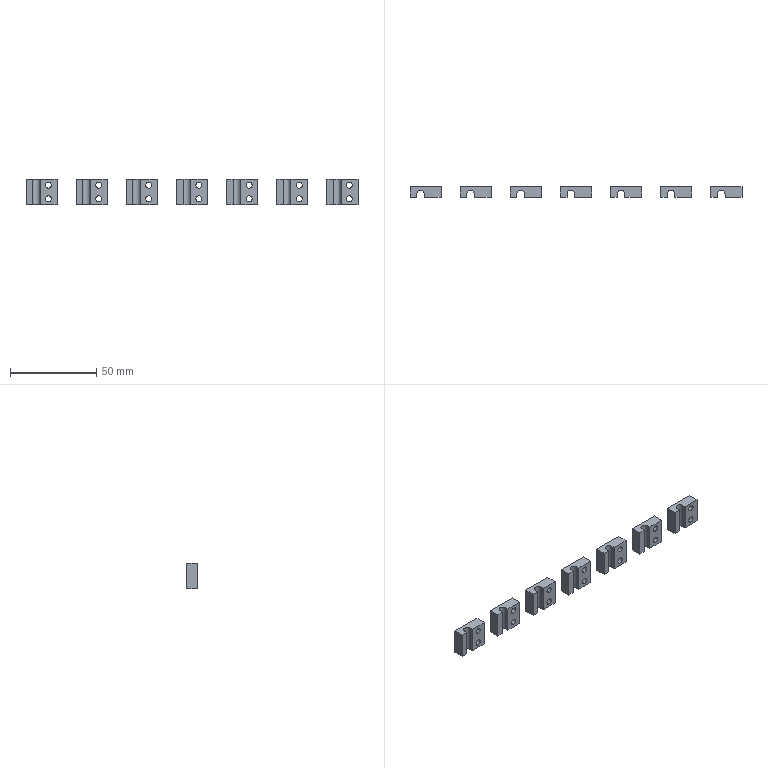NC program | Mastercam | posted with a generic post | part box 192 x 6 x 15 mm
Lines 1 to 1607 of 12453, first 1512 of 1607 lines:
%
:0001()
(MATERIAL - ALUMINUM MM - 2024)
(T20|63 FEM |H20)
(T9|10 FEM |H9|XY STOCK TO LEAVE - .1|Z STOCK TO LEAVE - 0.)
(T10|10 FEM |H10)
(T2|2 FEM |H2)
(T5|3 BM/BNOS |H5)
(T7|4 CHM |H7)
N100 G21
N102 G0 G17 G40 G80 G90 G94 G98
N104 G0 G28 G91 Z0.
N106 G0 G28 X0. Y0.
(63 FEM |TOOL - 20|DIA. OFF. - 20|LEN. - 20|TOOL DIA. - 63.)
N108 T20 M6
N110 G0 G54 G90 X-146.4 Y0. C0. B0. S4000 M3
N112 G43 H20 Z50.
N114 Z2.
N116 G1 Z0. F600.
N118 X146.4 F1000.
N120 G0 Z50.
N122 M5
N124 G0 G28 G91 Z0.
N126 G28
N128 M01
N130 G0 G17 G40 G80 G90 G94 G98
N132 G0 G28 G91 Z0.
(10 FEM |TOOL - 9|DIA. OFF. - 9|LEN. - 9|TOOL DIA. - 10.)
N134 T9 M6
N136 G0 G54 G90 X97. Y-18.6 C0. B0. S10000 M3
N138 G43 H9 Z50.
N140 Z1.
N142 G1 Z0. F600.
N144 Y-13.6 F4000.
N146 G3 X96. Y-12.6 I-1.
N148 G1 X78. Z-.092
N150 G2 X72.9 Y-7.5 Z-.133 J5.1
N152 G1 Y7.5 Z-.209
N154 G2 X78. Y12.6 Z-.25 I5.1
N156 G1 X96. Z-.342
N158 G2 X101.1 Y7.5 Z-.383 J-5.1
N160 G1 Y-7.5 Z-.459
N162 G2 X96. Y-12.6 Z-.5 I-5.1
N164 G1 X78. Z-.592
N166 G2 X72.9 Y-7.5 Z-.633 J5.1
N168 G1 Y7.5 Z-.709
N170 G2 X78. Y12.6 Z-.75 I5.1
N172 G1 X96. Z-.842
N174 G2 X101.1 Y7.5 Z-.883 J-5.1
N176 G1 Y-7.5 Z-.959
N178 G2 X96. Y-12.6 Z-1. I-5.1
N180 G1 X78. Z-1.092
N182 G2 X72.9 Y-7.5 Z-1.133 J5.1
N184 G1 Y7.5 Z-1.209
N186 G2 X78. Y12.6 Z-1.25 I5.1
N188 G1 X96. Z-1.342
N190 G2 X101.1 Y7.5 Z-1.383 J-5.1
N192 G1 Y-7.5 Z-1.459
N194 G2 X96. Y-12.6 Z-1.5 I-5.1
N196 G1 X78. Z-1.592
N198 G2 X72.9 Y-7.5 Z-1.633 J5.1
N200 G1 Y7.5 Z-1.709
N202 G2 X78. Y12.6 Z-1.75 I5.1
N204 G1 X96. Z-1.842
N206 G2 X101.1 Y7.5 Z-1.883 J-5.1
N208 G1 Y-7.5 Z-1.959
N210 G2 X96. Y-12.6 Z-2. I-5.1
N212 G1 X78. Z-2.092
N214 G2 X72.9 Y-7.5 Z-2.133 J5.1
N216 G1 Y7.5 Z-2.209
N218 G2 X78. Y12.6 Z-2.25 I5.1
N220 G1 X96. Z-2.342
N222 G2 X101.1 Y7.5 Z-2.383 J-5.1
N224 G1 Y-7.5 Z-2.459
N226 G2 X96. Y-12.6 Z-2.5 I-5.1
N228 G1 X78. Z-2.592
N230 G2 X72.9 Y-7.5 Z-2.633 J5.1
N232 G1 Y7.5 Z-2.709
N234 G2 X78. Y12.6 Z-2.75 I5.1
N236 G1 X96. Z-2.842
N238 G2 X101.1 Y7.5 Z-2.883 J-5.1
N240 G1 Y-7.5 Z-2.959
N242 G2 X96. Y-12.6 Z-3. I-5.1
N244 G1 X78. Z-3.092
N246 G2 X72.9 Y-7.5 Z-3.133 J5.1
N248 G1 Y7.5 Z-3.209
N250 G2 X78. Y12.6 Z-3.25 I5.1
N252 G1 X96. Z-3.342
N254 G2 X101.1 Y7.5 Z-3.383 J-5.1
N256 G1 Y-7.5 Z-3.459
N258 G2 X96. Y-12.6 Z-3.5 I-5.1
N260 G1 X78. Z-3.592
N262 G2 X72.9 Y-7.5 Z-3.633 J5.1
N264 G1 Y7.5 Z-3.709
N266 G2 X78. Y12.6 Z-3.75 I5.1
N268 G1 X96. Z-3.842
N270 G2 X101.1 Y7.5 Z-3.883 J-5.1
N272 G1 Y-7.5 Z-3.959
N274 G2 X96. Y-12.6 Z-4. I-5.1
N276 G1 X78. Z-4.092
N278 G2 X72.9 Y-7.5 Z-4.133 J5.1
N280 G1 Y7.5 Z-4.209
N282 G2 X78. Y12.6 Z-4.25 I5.1
N284 G1 X96. Z-4.342
N286 G2 X101.1 Y7.5 Z-4.383 J-5.1
N288 G1 Y-7.5 Z-4.459
N290 G2 X96. Y-12.6 Z-4.5 I-5.1
N292 G1 X78. Z-4.592
N294 G2 X72.9 Y-7.5 Z-4.633 J5.1
N296 G1 Y7.5 Z-4.709
N298 G2 X78. Y12.6 Z-4.75 I5.1
N300 G1 X96. Z-4.842
N302 G2 X101.1 Y7.5 Z-4.883 J-5.1
N304 G1 Y-7.5 Z-4.959
N306 G2 X96. Y-12.6 Z-5. I-5.1
N308 G1 X78. Z-5.092
N310 G2 X72.9 Y-7.5 Z-5.133 J5.1
N312 G1 Y7.5 Z-5.209
N314 G2 X78. Y12.6 Z-5.25 I5.1
N316 G1 X96. Z-5.342
N318 G2 X101.1 Y7.5 Z-5.383 J-5.1
N320 G1 Y-7.5 Z-5.459
N322 G2 X96. Y-12.6 Z-5.5 I-5.1
N324 G1 X78. Z-5.592
N326 G2 X72.9 Y-7.5 Z-5.633 J5.1
N328 G1 Y7.5 Z-5.709
N330 G2 X78. Y12.6 Z-5.75 I5.1
N332 G1 X96. Z-5.842
N334 G2 X101.1 Y7.5 Z-5.883 J-5.1
N336 G1 Y-7.5 Z-5.959
N338 G2 X96. Y-12.6 Z-6. I-5.1
N340 G1 X78. Z-6.092
N342 G2 X72.9 Y-7.5 Z-6.133 J5.1
N344 G1 Y7.5 Z-6.209
N346 G2 X78. Y12.6 Z-6.25 I5.1
N348 G1 X96. Z-6.342
N350 G2 X101.1 Y7.5 Z-6.383 J-5.1
N352 G1 Y-7.5 Z-6.459
N354 G2 X96. Y-12.6 Z-6.5 I-5.1
N356 G1 X78.
N358 G2 X72.9 Y-7.5 J5.1
N360 G1 Y7.5
N362 G2 X78. Y12.6 I5.1
N364 G1 X96.
N366 G2 X101.1 Y7.5 J-5.1
N368 G1 Y-7.5
N370 G2 X96. Y-12.6 I-5.1
N372 G1 X95.5
N374 G3 X94.5 Y-13.6 J-1.
N376 G1 Y-18.6
N378 G0 Z50.
N380 X68.
N382 Z1.
N384 G1 Z0. F600.
N386 Y-13.6 F4000.
N388 G3 X67. Y-12.6 I-1.
N390 G1 X49. Z-.092
N392 G2 X43.9 Y-7.5 Z-.133 J5.1
N394 G1 Y7.5 Z-.209
N396 G2 X49. Y12.6 Z-.25 I5.1
N398 G1 X67. Z-.342
N400 G2 X72.1 Y7.5 Z-.383 J-5.1
N402 G1 Y-7.5 Z-.459
N404 G2 X67. Y-12.6 Z-.5 I-5.1
N406 G1 X49. Z-.592
N408 G2 X43.9 Y-7.5 Z-.633 J5.1
N410 G1 Y7.5 Z-.709
N412 G2 X49. Y12.6 Z-.75 I5.1
N414 G1 X67. Z-.842
N416 G2 X72.1 Y7.5 Z-.883 J-5.1
N418 G1 Y-7.5 Z-.959
N420 G2 X67. Y-12.6 Z-1. I-5.1
N422 G1 X49. Z-1.092
N424 G2 X43.9 Y-7.5 Z-1.133 J5.1
N426 G1 Y7.5 Z-1.209
N428 G2 X49. Y12.6 Z-1.25 I5.1
N430 G1 X67. Z-1.342
N432 G2 X72.1 Y7.5 Z-1.383 J-5.1
N434 G1 Y-7.5 Z-1.459
N436 G2 X67. Y-12.6 Z-1.5 I-5.1
N438 G1 X49. Z-1.592
N440 G2 X43.9 Y-7.5 Z-1.633 J5.1
N442 G1 Y7.5 Z-1.709
N444 G2 X49. Y12.6 Z-1.75 I5.1
N446 G1 X67. Z-1.842
N448 G2 X72.1 Y7.5 Z-1.883 J-5.1
N450 G1 Y-7.5 Z-1.959
N452 G2 X67. Y-12.6 Z-2. I-5.1
N454 G1 X49. Z-2.092
N456 G2 X43.9 Y-7.5 Z-2.133 J5.1
N458 G1 Y7.5 Z-2.209
N460 G2 X49. Y12.6 Z-2.25 I5.1
N462 G1 X67. Z-2.342
N464 G2 X72.1 Y7.5 Z-2.383 J-5.1
N466 G1 Y-7.5 Z-2.459
N468 G2 X67. Y-12.6 Z-2.5 I-5.1
N470 G1 X49. Z-2.592
N472 G2 X43.9 Y-7.5 Z-2.633 J5.1
N474 G1 Y7.5 Z-2.709
N476 G2 X49. Y12.6 Z-2.75 I5.1
N478 G1 X67. Z-2.842
N480 G2 X72.1 Y7.5 Z-2.883 J-5.1
N482 G1 Y-7.5 Z-2.959
N484 G2 X67. Y-12.6 Z-3. I-5.1
N486 G1 X49. Z-3.092
N488 G2 X43.9 Y-7.5 Z-3.133 J5.1
N490 G1 Y7.5 Z-3.209
N492 G2 X49. Y12.6 Z-3.25 I5.1
N494 G1 X67. Z-3.342
N496 G2 X72.1 Y7.5 Z-3.383 J-5.1
N498 G1 Y-7.5 Z-3.459
N500 G2 X67. Y-12.6 Z-3.5 I-5.1
N502 G1 X49. Z-3.592
N504 G2 X43.9 Y-7.5 Z-3.633 J5.1
N506 G1 Y7.5 Z-3.709
N508 G2 X49. Y12.6 Z-3.75 I5.1
N510 G1 X67. Z-3.842
N512 G2 X72.1 Y7.5 Z-3.883 J-5.1
N514 G1 Y-7.5 Z-3.959
N516 G2 X67. Y-12.6 Z-4. I-5.1
N518 G1 X49. Z-4.092
N520 G2 X43.9 Y-7.5 Z-4.133 J5.1
N522 G1 Y7.5 Z-4.209
N524 G2 X49. Y12.6 Z-4.25 I5.1
N526 G1 X67. Z-4.342
N528 G2 X72.1 Y7.5 Z-4.383 J-5.1
N530 G1 Y-7.5 Z-4.459
N532 G2 X67. Y-12.6 Z-4.5 I-5.1
N534 G1 X49. Z-4.592
N536 G2 X43.9 Y-7.5 Z-4.633 J5.1
N538 G1 Y7.5 Z-4.709
N540 G2 X49. Y12.6 Z-4.75 I5.1
N542 G1 X67. Z-4.842
N544 G2 X72.1 Y7.5 Z-4.883 J-5.1
N546 G1 Y-7.5 Z-4.959
N548 G2 X67. Y-12.6 Z-5. I-5.1
N550 G1 X49. Z-5.092
N552 G2 X43.9 Y-7.5 Z-5.133 J5.1
N554 G1 Y7.5 Z-5.209
N556 G2 X49. Y12.6 Z-5.25 I5.1
N558 G1 X67. Z-5.342
N560 G2 X72.1 Y7.5 Z-5.383 J-5.1
N562 G1 Y-7.5 Z-5.459
N564 G2 X67. Y-12.6 Z-5.5 I-5.1
N566 G1 X49. Z-5.592
N568 G2 X43.9 Y-7.5 Z-5.633 J5.1
N570 G1 Y7.5 Z-5.709
N572 G2 X49. Y12.6 Z-5.75 I5.1
N574 G1 X67. Z-5.842
N576 G2 X72.1 Y7.5 Z-5.883 J-5.1
N578 G1 Y-7.5 Z-5.959
N580 G2 X67. Y-12.6 Z-6. I-5.1
N582 G1 X49. Z-6.092
N584 G2 X43.9 Y-7.5 Z-6.133 J5.1
N586 G1 Y7.5 Z-6.209
N588 G2 X49. Y12.6 Z-6.25 I5.1
N590 G1 X67. Z-6.342
N592 G2 X72.1 Y7.5 Z-6.383 J-5.1
N594 G1 Y-7.5 Z-6.459
N596 G2 X67. Y-12.6 Z-6.5 I-5.1
N598 G1 X49.
N600 G2 X43.9 Y-7.5 J5.1
N602 G1 Y7.5
N604 G2 X49. Y12.6 I5.1
N606 G1 X67.
N608 G2 X72.1 Y7.5 J-5.1
N610 G1 Y-7.5
N612 G2 X67. Y-12.6 I-5.1
N614 G1 X66.5
N616 G3 X65.5 Y-13.6 J-1.
N618 G1 Y-18.6
N620 G0 Z50.
N622 X39.
N624 Z1.
N626 G1 Z0. F600.
N628 Y-13.6 F4000.
N630 G3 X38. Y-12.6 I-1.
N632 G1 X20. Z-.092
N634 G2 X14.9 Y-7.5 Z-.133 J5.1
N636 G1 Y7.5 Z-.209
N638 G2 X20. Y12.6 Z-.25 I5.1
N640 G1 X38. Z-.342
N642 G2 X43.1 Y7.5 Z-.383 J-5.1
N644 G1 Y-7.5 Z-.459
N646 G2 X38. Y-12.6 Z-.5 I-5.1
N648 G1 X20. Z-.592
N650 G2 X14.9 Y-7.5 Z-.633 J5.1
N652 G1 Y7.5 Z-.709
N654 G2 X20. Y12.6 Z-.75 I5.1
N656 G1 X38. Z-.842
N658 G2 X43.1 Y7.5 Z-.883 J-5.1
N660 G1 Y-7.5 Z-.959
N662 G2 X38. Y-12.6 Z-1. I-5.1
N664 G1 X20. Z-1.092
N666 G2 X14.9 Y-7.5 Z-1.133 J5.1
N668 G1 Y7.5 Z-1.209
N670 G2 X20. Y12.6 Z-1.25 I5.1
N672 G1 X38. Z-1.342
N674 G2 X43.1 Y7.5 Z-1.383 J-5.1
N676 G1 Y-7.5 Z-1.459
N678 G2 X38. Y-12.6 Z-1.5 I-5.1
N680 G1 X20. Z-1.592
N682 G2 X14.9 Y-7.5 Z-1.633 J5.1
N684 G1 Y7.5 Z-1.709
N686 G2 X20. Y12.6 Z-1.75 I5.1
N688 G1 X38. Z-1.842
N690 G2 X43.1 Y7.5 Z-1.883 J-5.1
N692 G1 Y-7.5 Z-1.959
N694 G2 X38. Y-12.6 Z-2. I-5.1
N696 G1 X20. Z-2.092
N698 G2 X14.9 Y-7.5 Z-2.133 J5.1
N700 G1 Y7.5 Z-2.209
N702 G2 X20. Y12.6 Z-2.25 I5.1
N704 G1 X38. Z-2.342
N706 G2 X43.1 Y7.5 Z-2.383 J-5.1
N708 G1 Y-7.5 Z-2.459
N710 G2 X38. Y-12.6 Z-2.5 I-5.1
N712 G1 X20. Z-2.592
N714 G2 X14.9 Y-7.5 Z-2.633 J5.1
N716 G1 Y7.5 Z-2.709
N718 G2 X20. Y12.6 Z-2.75 I5.1
N720 G1 X38. Z-2.842
N722 G2 X43.1 Y7.5 Z-2.883 J-5.1
N724 G1 Y-7.5 Z-2.959
N726 G2 X38. Y-12.6 Z-3. I-5.1
N728 G1 X20. Z-3.092
N730 G2 X14.9 Y-7.5 Z-3.133 J5.1
N732 G1 Y7.5 Z-3.209
N734 G2 X20. Y12.6 Z-3.25 I5.1
N736 G1 X38. Z-3.342
N738 G2 X43.1 Y7.5 Z-3.383 J-5.1
N740 G1 Y-7.5 Z-3.459
N742 G2 X38. Y-12.6 Z-3.5 I-5.1
N744 G1 X20. Z-3.592
N746 G2 X14.9 Y-7.5 Z-3.633 J5.1
N748 G1 Y7.5 Z-3.709
N750 G2 X20. Y12.6 Z-3.75 I5.1
N752 G1 X38. Z-3.842
N754 G2 X43.1 Y7.5 Z-3.883 J-5.1
N756 G1 Y-7.5 Z-3.959
N758 G2 X38. Y-12.6 Z-4. I-5.1
N760 G1 X20. Z-4.092
N762 G2 X14.9 Y-7.5 Z-4.133 J5.1
N764 G1 Y7.5 Z-4.209
N766 G2 X20. Y12.6 Z-4.25 I5.1
N768 G1 X38. Z-4.342
N770 G2 X43.1 Y7.5 Z-4.383 J-5.1
N772 G1 Y-7.5 Z-4.459
N774 G2 X38. Y-12.6 Z-4.5 I-5.1
N776 G1 X20. Z-4.592
N778 G2 X14.9 Y-7.5 Z-4.633 J5.1
N780 G1 Y7.5 Z-4.709
N782 G2 X20. Y12.6 Z-4.75 I5.1
N784 G1 X38. Z-4.842
N786 G2 X43.1 Y7.5 Z-4.883 J-5.1
N788 G1 Y-7.5 Z-4.959
N790 G2 X38. Y-12.6 Z-5. I-5.1
N792 G1 X20. Z-5.092
N794 G2 X14.9 Y-7.5 Z-5.133 J5.1
N796 G1 Y7.5 Z-5.209
N798 G2 X20. Y12.6 Z-5.25 I5.1
N800 G1 X38. Z-5.342
N802 G2 X43.1 Y7.5 Z-5.383 J-5.1
N804 G1 Y-7.5 Z-5.459
N806 G2 X38. Y-12.6 Z-5.5 I-5.1
N808 G1 X20. Z-5.592
N810 G2 X14.9 Y-7.5 Z-5.633 J5.1
N812 G1 Y7.5 Z-5.709
N814 G2 X20. Y12.6 Z-5.75 I5.1
N816 G1 X38. Z-5.842
N818 G2 X43.1 Y7.5 Z-5.883 J-5.1
N820 G1 Y-7.5 Z-5.959
N822 G2 X38. Y-12.6 Z-6. I-5.1
N824 G1 X20. Z-6.092
N826 G2 X14.9 Y-7.5 Z-6.133 J5.1
N828 G1 Y7.5 Z-6.209
N830 G2 X20. Y12.6 Z-6.25 I5.1
N832 G1 X38. Z-6.342
N834 G2 X43.1 Y7.5 Z-6.383 J-5.1
N836 G1 Y-7.5 Z-6.459
N838 G2 X38. Y-12.6 Z-6.5 I-5.1
N840 G1 X20.
N842 G2 X14.9 Y-7.5 J5.1
N844 G1 Y7.5
N846 G2 X20. Y12.6 I5.1
N848 G1 X38.
N850 G2 X43.1 Y7.5 J-5.1
N852 G1 Y-7.5
N854 G2 X38. Y-12.6 I-5.1
N856 G1 X37.5
N858 G3 X36.5 Y-13.6 J-1.
N860 G1 Y-18.6
N862 G0 Z50.
N864 X10.
N866 Z1.
N868 G1 Z0. F600.
N870 Y-13.6 F4000.
N872 G3 X9. Y-12.6 I-1.
N874 G1 X-9. Z-.092
N876 G2 X-14.1 Y-7.5 Z-.133 J5.1
N878 G1 Y7.5 Z-.209
N880 G2 X-9. Y12.6 Z-.25 I5.1
N882 G1 X9. Z-.342
N884 G2 X14.1 Y7.5 Z-.383 J-5.1
N886 G1 Y-7.5 Z-.459
N888 G2 X9. Y-12.6 Z-.5 I-5.1
N890 G1 X-9. Z-.592
N892 G2 X-14.1 Y-7.5 Z-.633 J5.1
N894 G1 Y7.5 Z-.709
N896 G2 X-9. Y12.6 Z-.75 I5.1
N898 G1 X9. Z-.842
N900 G2 X14.1 Y7.5 Z-.883 J-5.1
N902 G1 Y-7.5 Z-.959
N904 G2 X9. Y-12.6 Z-1. I-5.1
N906 G1 X-9. Z-1.092
N908 G2 X-14.1 Y-7.5 Z-1.133 J5.1
N910 G1 Y7.5 Z-1.209
N912 G2 X-9. Y12.6 Z-1.25 I5.1
N914 G1 X9. Z-1.342
N916 G2 X14.1 Y7.5 Z-1.383 J-5.1
N918 G1 Y-7.5 Z-1.459
N920 G2 X9. Y-12.6 Z-1.5 I-5.1
N922 G1 X-9. Z-1.592
N924 G2 X-14.1 Y-7.5 Z-1.633 J5.1
N926 G1 Y7.5 Z-1.709
N928 G2 X-9. Y12.6 Z-1.75 I5.1
N930 G1 X9. Z-1.842
N932 G2 X14.1 Y7.5 Z-1.883 J-5.1
N934 G1 Y-7.5 Z-1.959
N936 G2 X9. Y-12.6 Z-2. I-5.1
N938 G1 X-9. Z-2.092
N940 G2 X-14.1 Y-7.5 Z-2.133 J5.1
N942 G1 Y7.5 Z-2.209
N944 G2 X-9. Y12.6 Z-2.25 I5.1
N946 G1 X9. Z-2.342
N948 G2 X14.1 Y7.5 Z-2.383 J-5.1
N950 G1 Y-7.5 Z-2.459
N952 G2 X9. Y-12.6 Z-2.5 I-5.1
N954 G1 X-9. Z-2.592
N956 G2 X-14.1 Y-7.5 Z-2.633 J5.1
N958 G1 Y7.5 Z-2.709
N960 G2 X-9. Y12.6 Z-2.75 I5.1
N962 G1 X9. Z-2.842
N964 G2 X14.1 Y7.5 Z-2.883 J-5.1
N966 G1 Y-7.5 Z-2.959
N968 G2 X9. Y-12.6 Z-3. I-5.1
N970 G1 X-9. Z-3.092
N972 G2 X-14.1 Y-7.5 Z-3.133 J5.1
N974 G1 Y7.5 Z-3.209
N976 G2 X-9. Y12.6 Z-3.25 I5.1
N978 G1 X9. Z-3.342
N980 G2 X14.1 Y7.5 Z-3.383 J-5.1
N982 G1 Y-7.5 Z-3.459
N984 G2 X9. Y-12.6 Z-3.5 I-5.1
N986 G1 X-9. Z-3.592
N988 G2 X-14.1 Y-7.5 Z-3.633 J5.1
N990 G1 Y7.5 Z-3.709
N992 G2 X-9. Y12.6 Z-3.75 I5.1
N994 G1 X9. Z-3.842
N996 G2 X14.1 Y7.5 Z-3.883 J-5.1
N998 G1 Y-7.5 Z-3.959
N1000 G2 X9. Y-12.6 Z-4. I-5.1
N1002 G1 X-9. Z-4.092
N1004 G2 X-14.1 Y-7.5 Z-4.133 J5.1
N1006 G1 Y7.5 Z-4.209
N1008 G2 X-9. Y12.6 Z-4.25 I5.1
N1010 G1 X9. Z-4.342
N1012 G2 X14.1 Y7.5 Z-4.383 J-5.1
N1014 G1 Y-7.5 Z-4.459
N1016 G2 X9. Y-12.6 Z-4.5 I-5.1
N1018 G1 X-9. Z-4.592
N1020 G2 X-14.1 Y-7.5 Z-4.633 J5.1
N1022 G1 Y7.5 Z-4.709
N1024 G2 X-9. Y12.6 Z-4.75 I5.1
N1026 G1 X9. Z-4.842
N1028 G2 X14.1 Y7.5 Z-4.883 J-5.1
N1030 G1 Y-7.5 Z-4.959
N1032 G2 X9. Y-12.6 Z-5. I-5.1
N1034 G1 X-9. Z-5.092
N1036 G2 X-14.1 Y-7.5 Z-5.133 J5.1
N1038 G1 Y7.5 Z-5.209
N1040 G2 X-9. Y12.6 Z-5.25 I5.1
N1042 G1 X9. Z-5.342
N1044 G2 X14.1 Y7.5 Z-5.383 J-5.1
N1046 G1 Y-7.5 Z-5.459
N1048 G2 X9. Y-12.6 Z-5.5 I-5.1
N1050 G1 X-9. Z-5.592
N1052 G2 X-14.1 Y-7.5 Z-5.633 J5.1
N1054 G1 Y7.5 Z-5.709
N1056 G2 X-9. Y12.6 Z-5.75 I5.1
N1058 G1 X9. Z-5.842
N1060 G2 X14.1 Y7.5 Z-5.883 J-5.1
N1062 G1 Y-7.5 Z-5.959
N1064 G2 X9. Y-12.6 Z-6. I-5.1
N1066 G1 X-9. Z-6.092
N1068 G2 X-14.1 Y-7.5 Z-6.133 J5.1
N1070 G1 Y7.5 Z-6.209
N1072 G2 X-9. Y12.6 Z-6.25 I5.1
N1074 G1 X9. Z-6.342
N1076 G2 X14.1 Y7.5 Z-6.383 J-5.1
N1078 G1 Y-7.5 Z-6.459
N1080 G2 X9. Y-12.6 Z-6.5 I-5.1
N1082 G1 X-9.
N1084 G2 X-14.1 Y-7.5 J5.1
N1086 G1 Y7.5
N1088 G2 X-9. Y12.6 I5.1
N1090 G1 X9.
N1092 G2 X14.1 Y7.5 J-5.1
N1094 G1 Y-7.5
N1096 G2 X9. Y-12.6 I-5.1
N1098 G1 X8.5
N1100 G3 X7.5 Y-13.6 J-1.
N1102 G1 Y-18.6
N1104 G0 Z50.
N1106 X-19.
N1108 Z1.
N1110 G1 Z0. F600.
N1112 Y-13.6 F4000.
N1114 G3 X-20. Y-12.6 I-1.
N1116 G1 X-38. Z-.092
N1118 G2 X-43.1 Y-7.5 Z-.133 J5.1
N1120 G1 Y7.5 Z-.209
N1122 G2 X-38. Y12.6 Z-.25 I5.1
N1124 G1 X-20. Z-.342
N1126 G2 X-14.9 Y7.5 Z-.383 J-5.1
N1128 G1 Y-7.5 Z-.459
N1130 G2 X-20. Y-12.6 Z-.5 I-5.1
N1132 G1 X-38. Z-.592
N1134 G2 X-43.1 Y-7.5 Z-.633 J5.1
N1136 G1 Y7.5 Z-.709
N1138 G2 X-38. Y12.6 Z-.75 I5.1
N1140 G1 X-20. Z-.842
N1142 G2 X-14.9 Y7.5 Z-.883 J-5.1
N1144 G1 Y-7.5 Z-.959
N1146 G2 X-20. Y-12.6 Z-1. I-5.1
N1148 G1 X-38. Z-1.092
N1150 G2 X-43.1 Y-7.5 Z-1.133 J5.1
N1152 G1 Y7.5 Z-1.209
N1154 G2 X-38. Y12.6 Z-1.25 I5.1
N1156 G1 X-20. Z-1.342
N1158 G2 X-14.9 Y7.5 Z-1.383 J-5.1
N1160 G1 Y-7.5 Z-1.459
N1162 G2 X-20. Y-12.6 Z-1.5 I-5.1
N1164 G1 X-38. Z-1.592
N1166 G2 X-43.1 Y-7.5 Z-1.633 J5.1
N1168 G1 Y7.5 Z-1.709
N1170 G2 X-38. Y12.6 Z-1.75 I5.1
N1172 G1 X-20. Z-1.842
N1174 G2 X-14.9 Y7.5 Z-1.883 J-5.1
N1176 G1 Y-7.5 Z-1.959
N1178 G2 X-20. Y-12.6 Z-2. I-5.1
N1180 G1 X-38. Z-2.092
N1182 G2 X-43.1 Y-7.5 Z-2.133 J5.1
N1184 G1 Y7.5 Z-2.209
N1186 G2 X-38. Y12.6 Z-2.25 I5.1
N1188 G1 X-20. Z-2.342
N1190 G2 X-14.9 Y7.5 Z-2.383 J-5.1
N1192 G1 Y-7.5 Z-2.459
N1194 G2 X-20. Y-12.6 Z-2.5 I-5.1
N1196 G1 X-38. Z-2.592
N1198 G2 X-43.1 Y-7.5 Z-2.633 J5.1
N1200 G1 Y7.5 Z-2.709
N1202 G2 X-38. Y12.6 Z-2.75 I5.1
N1204 G1 X-20. Z-2.842
N1206 G2 X-14.9 Y7.5 Z-2.883 J-5.1
N1208 G1 Y-7.5 Z-2.959
N1210 G2 X-20. Y-12.6 Z-3. I-5.1
N1212 G1 X-38. Z-3.092
N1214 G2 X-43.1 Y-7.5 Z-3.133 J5.1
N1216 G1 Y7.5 Z-3.209
N1218 G2 X-38. Y12.6 Z-3.25 I5.1
N1220 G1 X-20. Z-3.342
N1222 G2 X-14.9 Y7.5 Z-3.383 J-5.1
N1224 G1 Y-7.5 Z-3.459
N1226 G2 X-20. Y-12.6 Z-3.5 I-5.1
N1228 G1 X-38. Z-3.592
N1230 G2 X-43.1 Y-7.5 Z-3.633 J5.1
N1232 G1 Y7.5 Z-3.709
N1234 G2 X-38. Y12.6 Z-3.75 I5.1
N1236 G1 X-20. Z-3.842
N1238 G2 X-14.9 Y7.5 Z-3.883 J-5.1
N1240 G1 Y-7.5 Z-3.959
N1242 G2 X-20. Y-12.6 Z-4. I-5.1
N1244 G1 X-38. Z-4.092
N1246 G2 X-43.1 Y-7.5 Z-4.133 J5.1
N1248 G1 Y7.5 Z-4.209
N1250 G2 X-38. Y12.6 Z-4.25 I5.1
N1252 G1 X-20. Z-4.342
N1254 G2 X-14.9 Y7.5 Z-4.383 J-5.1
N1256 G1 Y-7.5 Z-4.459
N1258 G2 X-20. Y-12.6 Z-4.5 I-5.1
N1260 G1 X-38. Z-4.592
N1262 G2 X-43.1 Y-7.5 Z-4.633 J5.1
N1264 G1 Y7.5 Z-4.709
N1266 G2 X-38. Y12.6 Z-4.75 I5.1
N1268 G1 X-20. Z-4.842
N1270 G2 X-14.9 Y7.5 Z-4.883 J-5.1
N1272 G1 Y-7.5 Z-4.959
N1274 G2 X-20. Y-12.6 Z-5. I-5.1
N1276 G1 X-38. Z-5.092
N1278 G2 X-43.1 Y-7.5 Z-5.133 J5.1
N1280 G1 Y7.5 Z-5.209
N1282 G2 X-38. Y12.6 Z-5.25 I5.1
N1284 G1 X-20. Z-5.342
N1286 G2 X-14.9 Y7.5 Z-5.383 J-5.1
N1288 G1 Y-7.5 Z-5.459
N1290 G2 X-20. Y-12.6 Z-5.5 I-5.1
N1292 G1 X-38. Z-5.592
N1294 G2 X-43.1 Y-7.5 Z-5.633 J5.1
N1296 G1 Y7.5 Z-5.709
N1298 G2 X-38. Y12.6 Z-5.75 I5.1
N1300 G1 X-20. Z-5.842
N1302 G2 X-14.9 Y7.5 Z-5.883 J-5.1
N1304 G1 Y-7.5 Z-5.959
N1306 G2 X-20. Y-12.6 Z-6. I-5.1
N1308 G1 X-38. Z-6.092
N1310 G2 X-43.1 Y-7.5 Z-6.133 J5.1
N1312 G1 Y7.5 Z-6.209
N1314 G2 X-38. Y12.6 Z-6.25 I5.1
N1316 G1 X-20. Z-6.342
N1318 G2 X-14.9 Y7.5 Z-6.383 J-5.1
N1320 G1 Y-7.5 Z-6.459
N1322 G2 X-20. Y-12.6 Z-6.5 I-5.1
N1324 G1 X-38.
N1326 G2 X-43.1 Y-7.5 J5.1
N1328 G1 Y7.5
N1330 G2 X-38. Y12.6 I5.1
N1332 G1 X-20.
N1334 G2 X-14.9 Y7.5 J-5.1
N1336 G1 Y-7.5
N1338 G2 X-20. Y-12.6 I-5.1
N1340 G1 X-20.5
N1342 G3 X-21.5 Y-13.6 J-1.
N1344 G1 Y-18.6
N1346 G0 Z50.
N1348 X-48.
N1350 Z1.
N1352 G1 Z0. F600.
N1354 Y-13.6 F4000.
N1356 G3 X-49. Y-12.6 I-1.
N1358 G1 X-67. Z-.092
N1360 G2 X-72.1 Y-7.5 Z-.133 J5.1
N1362 G1 Y7.5 Z-.209
N1364 G2 X-67. Y12.6 Z-.25 I5.1
N1366 G1 X-49. Z-.342
N1368 G2 X-43.9 Y7.5 Z-.383 J-5.1
N1370 G1 Y-7.5 Z-.459
N1372 G2 X-49. Y-12.6 Z-.5 I-5.1
N1374 G1 X-67. Z-.592
N1376 G2 X-72.1 Y-7.5 Z-.633 J5.1
N1378 G1 Y7.5 Z-.709
N1380 G2 X-67. Y12.6 Z-.75 I5.1
N1382 G1 X-49. Z-.842
N1384 G2 X-43.9 Y7.5 Z-.883 J-5.1
N1386 G1 Y-7.5 Z-.959
N1388 G2 X-49. Y-12.6 Z-1. I-5.1
N1390 G1 X-67. Z-1.092
N1392 G2 X-72.1 Y-7.5 Z-1.133 J5.1
N1394 G1 Y7.5 Z-1.209
N1396 G2 X-67. Y12.6 Z-1.25 I5.1
N1398 G1 X-49. Z-1.342
N1400 G2 X-43.9 Y7.5 Z-1.383 J-5.1
N1402 G1 Y-7.5 Z-1.459
N1404 G2 X-49. Y-12.6 Z-1.5 I-5.1
N1406 G1 X-67. Z-1.592
N1408 G2 X-72.1 Y-7.5 Z-1.633 J5.1
N1410 G1 Y7.5 Z-1.709
N1412 G2 X-67. Y12.6 Z-1.75 I5.1
N1414 G1 X-49. Z-1.842
N1416 G2 X-43.9 Y7.5 Z-1.883 J-5.1
N1418 G1 Y-7.5 Z-1.959
N1420 G2 X-49. Y-12.6 Z-2. I-5.1
N1422 G1 X-67. Z-2.092
N1424 G2 X-72.1 Y-7.5 Z-2.133 J5.1
N1426 G1 Y7.5 Z-2.209
N1428 G2 X-67. Y12.6 Z-2.25 I5.1
N1430 G1 X-49. Z-2.342
N1432 G2 X-43.9 Y7.5 Z-2.383 J-5.1
N1434 G1 Y-7.5 Z-2.459
N1436 G2 X-49. Y-12.6 Z-2.5 I-5.1
N1438 G1 X-67. Z-2.592
N1440 G2 X-72.1 Y-7.5 Z-2.633 J5.1
N1442 G1 Y7.5 Z-2.709
N1444 G2 X-67. Y12.6 Z-2.75 I5.1
N1446 G1 X-49. Z-2.842
N1448 G2 X-43.9 Y7.5 Z-2.883 J-5.1
N1450 G1 Y-7.5 Z-2.959
N1452 G2 X-49. Y-12.6 Z-3. I-5.1
N1454 G1 X-67. Z-3.092
N1456 G2 X-72.1 Y-7.5 Z-3.133 J5.1
N1458 G1 Y7.5 Z-3.209
N1460 G2 X-67. Y12.6 Z-3.25 I5.1
N1462 G1 X-49. Z-3.342
N1464 G2 X-43.9 Y7.5 Z-3.383 J-5.1
N1466 G1 Y-7.5 Z-3.459
N1468 G2 X-49. Y-12.6 Z-3.5 I-5.1
N1470 G1 X-67. Z-3.592
N1472 G2 X-72.1 Y-7.5 Z-3.633 J5.1
N1474 G1 Y7.5 Z-3.709
N1476 G2 X-67. Y12.6 Z-3.75 I5.1
N1478 G1 X-49. Z-3.842
N1480 G2 X-43.9 Y7.5 Z-3.883 J-5.1
N1482 G1 Y-7.5 Z-3.959
N1484 G2 X-49. Y-12.6 Z-4. I-5.1
N1486 G1 X-67. Z-4.092
N1488 G2 X-72.1 Y-7.5 Z-4.133 J5.1
N1490 G1 Y7.5 Z-4.209
N1492 G2 X-67. Y12.6 Z-4.25 I5.1
N1494 G1 X-49. Z-4.342
N1496 G2 X-43.9 Y7.5 Z-4.383 J-5.1
N1498 G1 Y-7.5 Z-4.459
N1500 G2 X-49. Y-12.6 Z-4.5 I-5.1
N1502 G1 X-67. Z-4.592
N1504 G2 X-72.1 Y-7.5 Z-4.633 J5.1
N1506 G1 Y7.5 Z-4.709
N1508 G2 X-67. Y12.6 Z-4.75 I5.1
N1510 G1 X-49. Z-4.842
N1512 G2 X-43.9 Y7.5 Z-4.883 J-5.1
N1514 G1 Y-7.5 Z-4.959
N1516 G2 X-49. Y-12.6 Z-5. I-5.1
N1518 G1 X-67. Z-5.092
N1520 G2 X-72.1 Y-7.5 Z-5.133 J5.1
N1522 G1 Y7.5 Z-5.209
N1524 G2 X-67. Y12.6 Z-5.25 I5.1
N1526 G1 X-49. Z-5.342
N1528 G2 X-43.9 Y7.5 Z-5.383 J-5.1
N1530 G1 Y-7.5 Z-5.459
N1532 G2 X-49. Y-12.6 Z-5.5 I-5.1
N1534 G1 X-67. Z-5.592
N1536 G2 X-72.1 Y-7.5 Z-5.633 J5.1
N1538 G1 Y7.5 Z-5.709
N1540 G2 X-67. Y12.6 Z-5.75 I5.1
N1542 G1 X-49. Z-5.842
N1544 G2 X-43.9 Y7.5 Z-5.883 J-5.1
N1546 G1 Y-7.5 Z-5.959
N1548 G2 X-49. Y-12.6 Z-6. I-5.1
N1550 G1 X-67. Z-6.092
N1552 G2 X-72.1 Y-7.5 Z-6.133 J5.1
N1554 G1 Y7.5 Z-6.209
N1556 G2 X-67. Y12.6 Z-6.25 I5.1
N1558 G1 X-49. Z-6.342
N1560 G2 X-43.9 Y7.5 Z-6.383 J-5.1
N1562 G1 Y-7.5 Z-6.459
N1564 G2 X-49. Y-12.6 Z-6.5 I-5.1
N1566 G1 X-67.
N1568 G2 X-72.1 Y-7.5 J5.1
N1570 G1 Y7.5
N1572 G2 X-67. Y12.6 I5.1
N1574 G1 X-49.
N1576 G2 X-43.9 Y7.5 J-5.1
N1578 G1 Y-7.5
N1580 G2 X-49. Y-12.6 I-5.1
N1582 G1 X-49.5
N1584 G3 X-50.5 Y-13.6 J-1.
N1586 G1 Y-18.6
N1588 G0 Z50.
N1590 X-77.
N1592 Z1.
N1594 G1 Z0. F600.
N1596 Y-13.6 F4000.
N1598 G3 X-78. Y-12.6 I-1.
N1600 G1 X-96. Z-.092
N1602 G2 X-101.1 Y-7.5 Z-.133 J5.1
N1604 G1 Y7.5 Z-.209
N1606 G2 X-96. Y12.6 Z-.25 I5.1
N1608 G1 X-78. Z-.342
N1610 G2 X-72.9 Y7.5 Z-.383 J-5.1
N1612 G1 Y-7.5 Z-.459
N1614 G2 X-78. Y-12.6 Z-.5 I-5.1
N1616 G1 X-96. Z-.592
N1618 G2 X-101.1 Y-7.5 Z-.633 J5.1
N1620 G1 Y7.5 Z-.709
N1622 G2 X-96. Y12.6 Z-.75 I5.1
N1624 G1 X-78. Z-.842
N1626 G2 X-72.9 Y7.5 Z-.883 J-5.1
N1628 G1 Y-7.5 Z-.959
N1630 G2 X-78. Y-12.6 Z-1. I-5.1
N1632 G1 X-96. Z-1.092
N1634 G2 X-101.1 Y-7.5 Z-1.133 J5.1
N1636 G1 Y7.5 Z-1.209
N1638 G2 X-96. Y12.6 Z-1.25 I5.1
N1640 G1 X-78. Z-1.342
N1642 G2 X-72.9 Y7.5 Z-1.383 J-5.1
N1644 G1 Y-7.5 Z-1.459
N1646 G2 X-78. Y-12.6 Z-1.5 I-5.1
N1648 G1 X-96. Z-1.592
N1650 G2 X-101.1 Y-7.5 Z-1.633 J5.1
N1652 G1 Y7.5 Z-1.709
N1654 G2 X-96. Y12.6 Z-1.75 I5.1
N1656 G1 X-78. Z-1.842
N1658 G2 X-72.9 Y7.5 Z-1.883 J-5.1
N1660 G1 Y-7.5 Z-1.959
N1662 G2 X-78. Y-12.6 Z-2. I-5.1
N1664 G1 X-96. Z-2.092
N1666 G2 X-101.1 Y-7.5 Z-2.133 J5.1
N1668 G1 Y7.5 Z-2.209
N1670 G2 X-96. Y12.6 Z-2.25 I5.1
N1672 G1 X-78. Z-2.342
N1674 G2 X-72.9 Y7.5 Z-2.383 J-5.1
N1676 G1 Y-7.5 Z-2.459
N1678 G2 X-78. Y-12.6 Z-2.5 I-5.1
N1680 G1 X-96. Z-2.592
N1682 G2 X-101.1 Y-7.5 Z-2.633 J5.1
N1684 G1 Y7.5 Z-2.709
N1686 G2 X-96. Y12.6 Z-2.75 I5.1
N1688 G1 X-78. Z-2.842
N1690 G2 X-72.9 Y7.5 Z-2.883 J-5.1
N1692 G1 Y-7.5 Z-2.959
N1694 G2 X-78. Y-12.6 Z-3. I-5.1
N1696 G1 X-96. Z-3.092
N1698 G2 X-101.1 Y-7.5 Z-3.133 J5.1
N1700 G1 Y7.5 Z-3.209
N1702 G2 X-96. Y12.6 Z-3.25 I5.1
N1704 G1 X-78. Z-3.342
N1706 G2 X-72.9 Y7.5 Z-3.383 J-5.1
N1708 G1 Y-7.5 Z-3.459
N1710 G2 X-78. Y-12.6 Z-3.5 I-5.1
N1712 G1 X-96. Z-3.592
N1714 G2 X-101.1 Y-7.5 Z-3.633 J5.1
N1716 G1 Y7.5 Z-3.709
N1718 G2 X-96. Y12.6 Z-3.75 I5.1
N1720 G1 X-78. Z-3.842
N1722 G2 X-72.9 Y7.5 Z-3.883 J-5.1
N1724 G1 Y-7.5 Z-3.959
N1726 G2 X-78. Y-12.6 Z-4. I-5.1
N1728 G1 X-96. Z-4.092
N1730 G2 X-101.1 Y-7.5 Z-4.133 J5.1
N1732 G1 Y7.5 Z-4.209
N1734 G2 X-96. Y12.6 Z-4.25 I5.1
N1736 G1 X-78. Z-4.342
N1738 G2 X-72.9 Y7.5 Z-4.383 J-5.1
N1740 G1 Y-7.5 Z-4.459
N1742 G2 X-78. Y-12.6 Z-4.5 I-5.1
N1744 G1 X-96. Z-4.592
N1746 G2 X-101.1 Y-7.5 Z-4.633 J5.1
N1748 G1 Y7.5 Z-4.709
N1750 G2 X-96. Y12.6 Z-4.75 I5.1
N1752 G1 X-78. Z-4.842
N1754 G2 X-72.9 Y7.5 Z-4.883 J-5.1
N1756 G1 Y-7.5 Z-4.959
N1758 G2 X-78. Y-12.6 Z-5. I-5.1
N1760 G1 X-96. Z-5.092
N1762 G2 X-101.1 Y-7.5 Z-5.133 J5.1
N1764 G1 Y7.5 Z-5.209
N1766 G2 X-96. Y12.6 Z-5.25 I5.1
N1768 G1 X-78. Z-5.342
N1770 G2 X-72.9 Y7.5 Z-5.383 J-5.1
N1772 G1 Y-7.5 Z-5.459
N1774 G2 X-78. Y-12.6 Z-5.5 I-5.1
N1776 G1 X-96. Z-5.592
N1778 G2 X-101.1 Y-7.5 Z-5.633 J5.1
N1780 G1 Y7.5 Z-5.709
N1782 G2 X-96. Y12.6 Z-5.75 I5.1
N1784 G1 X-78. Z-5.842
N1786 G2 X-72.9 Y7.5 Z-5.883 J-5.1
N1788 G1 Y-7.5 Z-5.959
N1790 G2 X-78. Y-12.6 Z-6. I-5.1
N1792 G1 X-96. Z-6.092
N1794 G2 X-101.1 Y-7.5 Z-6.133 J5.1
N1796 G1 Y7.5 Z-6.209
N1798 G2 X-96. Y12.6 Z-6.25 I5.1
N1800 G1 X-78. Z-6.342
N1802 G2 X-72.9 Y7.5 Z-6.383 J-5.1
N1804 G1 Y-7.5 Z-6.459
N1806 G2 X-78. Y-12.6 Z-6.5 I-5.1
N1808 G1 X-96.
N1810 G2 X-101.1 Y-7.5 J5.1
N1812 G1 Y7.5
N1814 G2 X-96. Y12.6 I5.1
N1816 G1 X-78.
N1818 G2 X-72.9 Y7.5 J-5.1
N1820 G1 Y-7.5
N1822 G2 X-78. Y-12.6 I-5.1
N1824 G1 X-78.5
N1826 G3 X-79.5 Y-13.6 J-1.
N1828 G1 Y-18.6
N1830 G0 Z50.
N1832 M5
N1834 G0 G28 G91 Z0.
N1836 G28
N1838 M01
N1840 G0 G17 G40 G80 G90 G94 G98
N1842 G0 G28 G91 Z0.
(10 FEM |TOOL - 10|DIA. OFF. - 10|LEN. - 10|TOOL DIA. - 10.)
N1844 T10 M6
N1846 G0 G54 G90 X88. Y-15.5 C0. B0. S8000 M3
N1848 G43 H10 Z50.
N1850 Z1.
N1852 G1 Z-6.5 F600.
N1854 Y-13.5 F1000.
N1856 G3 X87. Y-12.5 I-1.
N1858 G1 X78.
N1860 G2 X73. Y-7.5 J5.
N1862 G1 Y7.5
N1864 G2 X78. Y12.5 I5.
N1866 G1 X96.
N1868 G2 X101. Y7.5 J-5.
N1870 G1 Y-7.5
N1872 G2 X96. Y-12.5 I-5.
N1874 G1 X87.
N1876 X86.5
N1878 G3 X85.5 Y-13.5 J-1.
N1880 G1 Y-15.5
N1882 G0 Z50.
N1884 X59.
N1886 Z1.
N1888 G1 Z-6.5 F600.
N1890 Y-13.5 F1000.
N1892 G3 X58. Y-12.5 I-1.
N1894 G1 X49.
N1896 G2 X44. Y-7.5 J5.
N1898 G1 Y7.5
N1900 G2 X49. Y12.5 I5.
N1902 G1 X67.
N1904 G2 X72. Y7.5 J-5.
N1906 G1 Y-7.5
N1908 G2 X67. Y-12.5 I-5.
N1910 G1 X58.
N1912 X57.5
N1914 G3 X56.5 Y-13.5 J-1.
N1916 G1 Y-15.5
N1918 G0 Z50.
N1920 X30.
N1922 Z1.
N1924 G1 Z-6.5 F600.
N1926 Y-13.5 F1000.
N1928 G3 X29. Y-12.5 I-1.
N1930 G1 X20.
N1932 G2 X15. Y-7.5 J5.
N1934 G1 Y7.5
N1936 G2 X20. Y12.5 I5.
N1938 G1 X38.
N1940 G2 X43. Y7.5 J-5.
N1942 G1 Y-7.5
N1944 G2 X38. Y-12.5 I-5.
N1946 G1 X29.
N1948 X28.5
N1950 G3 X27.5 Y-13.5 J-1.
N1952 G1 Y-15.5
N1954 G0 Z50.
N1956 X1.
N1958 Z1.
N1960 G1 Z-6.5 F600.
N1962 Y-13.5 F1000.
N1964 G3 X0. Y-12.5 I-1.
N1966 G1 X-9.
N1968 G2 X-14. Y-7.5 J5.
N1970 G1 Y7.5
N1972 G2 X-9. Y12.5 I5.
N1974 G1 X9.
N1976 G2 X14. Y7.5 J-5.
N1978 G1 Y-7.5
N1980 G2 X9. Y-12.5 I-5.
N1982 G1 X0.
N1984 X-.5
N1986 G3 X-1.5 Y-13.5 J-1.
N1988 G1 Y-15.5
N1990 G0 Z50.
N1992 X-28.
N1994 Z1.
N1996 G1 Z-6.5 F600.
N1998 Y-13.5 F1000.
N2000 G3 X-29. Y-12.5 I-1.
N2002 G1 X-38.
N2004 G2 X-43. Y-7.5 J5.
N2006 G1 Y7.5
N2008 G2 X-38. Y12.5 I5.
N2010 G1 X-20.
N2012 G2 X-15. Y7.5 J-5.
N2014 G1 Y-7.5
N2016 G2 X-20. Y-12.5 I-5.
N2018 G1 X-29.
N2020 X-29.5
N2022 G3 X-30.5 Y-13.5 J-1.
N2024 G1 Y-15.5
N2026 G0 Z50.
N2028 X-57.
N2030 Z1.
N2032 G1 Z-6.5 F600.
N2034 Y-13.5 F1000.
N2036 G3 X-58. Y-12.5 I-1.
N2038 G1 X-67.
N2040 G2 X-72. Y-7.5 J5.
N2042 G1 Y7.5
N2044 G2 X-67. Y12.5 I5.
N2046 G1 X-49.
N2048 G2 X-44. Y7.5 J-5.
N2050 G1 Y-7.5
N2052 G2 X-49. Y-12.5 I-5.
N2054 G1 X-58.
N2056 X-58.5
N2058 G3 X-59.5 Y-13.5 J-1.
N2060 G1 Y-15.5
N2062 G0 Z50.
N2064 X-86.
N2066 Z1.
N2068 G1 Z-6.5 F600.
N2070 Y-13.5 F1000.
N2072 G3 X-87. Y-12.5 I-1.
N2074 G1 X-96.
N2076 G2 X-101. Y-7.5 J5.
N2078 G1 Y7.5
N2080 G2 X-96. Y12.5 I5.
N2082 G1 X-78.
N2084 G2 X-73. Y7.5 J-5.
N2086 G1 Y-7.5
N2088 G2 X-78. Y-12.5 I-5.
N2090 G1 X-87.
N2092 X-87.5
N2094 G3 X-88.5 Y-13.5 J-1.
N2096 G1 Y-15.5
N2098 G0 Z50.
N2100 M5
N2102 G0 G28 G91 Z0.
N2104 G28
N2106 M01
N2108 G0 G17 G40 G80 G90 G94 G98
N2110 G0 G28 G91 Z0.
(2 FEM |TOOL - 2|DIA. OFF. - 2|LEN. - 2|TOOL DIA. - 2.)
N2112 T2 M6
N2114 G0 G54 G90 X-94. Y1.856 C0. B0. S7000 M3
N2116 G43 H2 Z50.
N2118 Z3.61
N2120 G1 Z3.11 F600.
N2122 X-93.989 Z2.901 F3000.
N2124 X-93.957 Z2.694
N2126 X-93.902 Z2.492
N2128 X-93.827 Z2.296
N2130 X-93.732 Z2.11
N2132 X-93.618 Z1.934
N2134 X-93.487 Z1.771
N2136 X-93.338 Z1.623
N2138 X-93.176 Z1.492
N2140 X-93. Z1.378
N2142 X-92.814 Z1.283
N2144 X-92.618 Z1.208
N2146 X-92.416 Z1.153
N2148 X-92.209 Z1.121
N2150 X-92. Z1.11
N2152 G2 X-90. Y-.144 Z1. J-2.
N2154 G1 Y-1.244 Z.981
N2156 Y-2.344 Z.962
N2158 Y-3.444 Z.943
N2160 Y-4.544 Z.924
N2162 Y-6.4 Z.905
N2164 Y-5.644
N2166 Y-4.544 Z.886
N2168 Y-3.444 Z.867
N2170 Y-2.344 Z.848
N2172 Y-1.244 Z.83
N2174 Y-.144 Z.811
N2176 Y0. Z.808
N2178 Y.956 Z.792
N2180 Y2.056 Z.773
N2182 Y3.156 Z.754
N2184 Y4.256 Z.735
N2186 Y6.4 Z.716
N2188 Y5.356
N2190 Y4.256 Z.697
N2192 Y3.156 Z.678
N2194 Y2.056 Z.659
N2196 Y.956 Z.64
N2198 Y-.144 Z.621
N2200 Y-1.244 Z.602
N2202 Y-2.344 Z.583
N2204 Y-3.444 Z.564
N2206 Y-4.544 Z.545
N2208 Y-6.4 Z.527
N2210 Y-5.644
N2212 Y-4.544 Z.508
N2214 Y-3.444 Z.489
N2216 Y-2.344 Z.47
N2218 Y-1.244 Z.451
N2220 Y-.144 Z.432
N2222 Y0. Z.429
N2224 Y.956 Z.413
N2226 Y2.056 Z.394
N2228 Y3.156 Z.375
N2230 Y4.256 Z.356
N2232 Y6.4 Z.337
N2234 Y5.356
N2236 Y4.256 Z.318
N2238 Y3.156 Z.299
N2240 Y2.056 Z.28
N2242 Y.956 Z.261
N2244 Y-.144 Z.242
N2246 Y-1.244 Z.223
N2248 Y-2.344 Z.205
N2250 Y-3.444 Z.186
N2252 Y-4.544 Z.167
N2254 Y-6.4 Z.148
N2256 Y-5.644
N2258 Y-4.544 Z.129
N2260 Y-3.444 Z.11
N2262 Y-2.344 Z.091
N2264 Y-1.244 Z.072
N2266 Y-.144 Z.053
N2268 Y0. Z.051
N2270 Y.956 Z.034
N2272 Y2.056 Z.015
N2274 Y3.156 Z-.004
N2276 Y4.256 Z-.023
N2278 Y6.4 Z-.042
N2280 Y5.356
N2282 Y4.256 Z-.061
N2284 Y3.156 Z-.08
N2286 Y2.056 Z-.098
N2288 Y.956 Z-.117
N2290 Y-.144 Z-.136
N2292 Y-1.244 Z-.155
N2294 Y-2.344 Z-.174
N2296 Y-3.444 Z-.193
N2298 Y-4.544 Z-.212
N2300 Y-6.4 Z-.231
N2302 Y-5.644
N2304 Y-4.544 Z-.25
N2306 Y0.
N2308 Y6.4
N2310 Y-6.4
N2312 Y-4.544
N2314 G2 X-89.849 Y-4.346 I.206
N2316 G1 X-89.051 Y-4.124
N2318 G3 X-88.9 Y-3.926 I-.055 J.198
N2320 G1 Y0.
N2322 Y7.5
N2324 X-91.1
N2326 Y-7.5
N2328 X-88.9
N2330 Y-3.926
N2332 G3 X-88.902 Y-3.894 I-.206
N2334 G1 X-89.997 Y3.262
N2336 G2 X-90. Y3.293 I.203 J.031
N2338 G1 Y4.393 Z-.268
N2340 Y6.4 Z-.286
N2342 Y5.493
N2344 Y4.393 Z-.304
N2346 Y3.293 Z-.321
N2348 Y2.193 Z-.339
N2350 Y1.093 Z-.357
N2352 Y-.007 Z-.375
N2354 Y-1.107 Z-.393
N2356 Y-2.207 Z-.411
N2358 Y-3.307 Z-.429
N2360 Y-4.407 Z-.446
N2362 Y-6.4 Z-.464
N2364 Y-5.507
N2366 Y-4.407 Z-.482
N2368 Y-3.307 Z-.5
N2370 Y0.
N2372 Y6.4
N2374 Y-6.4
N2376 Y-3.307
N2378 G2 X-89.849 Y-3.108 I.206
N2380 G1 X-89.051 Y-2.887
N2382 G3 X-88.9 Y-2.688 I-.055 J.199
N2384 G1 Y0.
N2386 Y7.5
N2388 X-91.1
N2390 Y-7.5
N2392 X-88.9
N2394 Y-2.688
N2396 G3 X-88.902 Y-2.657 I-.206
N2398 G1 X-89.997 Y4.499
N2400 G2 X-90. Y4.531 I.203 J.032
N2402 G1 Y6.4 Z-.518
N2404 Y5.631
N2406 Y4.531 Z-.536
N2408 Y3.431 Z-.554
N2410 Y2.331 Z-.571
N2412 Y1.231 Z-.589
N2414 Y.131 Z-.607
N2416 Y-.969 Z-.625
N2418 Y-2.069 Z-.643
N2420 Y-3.169 Z-.661
N2422 Y-4.269 Z-.679
N2424 Y-6.4 Z-.696
N2426 Y-5.369
N2428 Y-4.269 Z-.714
N2430 Y-3.169 Z-.732
N2432 Y-2.069 Z-.75
N2434 Y0.
N2436 Y6.4
N2438 Y-6.4
N2440 Y-2.069
N2442 G2 X-89.849 Y-1.871 I.206
N2444 G1 X-89.051 Y-1.649
N2446 G3 X-88.9 Y-1.451 I-.055 J.198
N2448 G1 Y0.
N2450 Y7.5
N2452 X-91.1
N2454 Y-7.5
N2456 X-88.9
N2458 Y-1.451
N2460 G3 X-88.902 Y-1.423 I-.206
N2462 G1 X-89.59 Y3.596
N2464 G3 X-89.794 Y3.774 I-.204 J-.028
N2466 X-90. Y3.568 J-.206
N2468 G1 Y2.468 Z-.768
N2470 Y1.368 Z-.786
N2472 Y.268 Z-.804
N2474 Y-.832 Z-.821
N2476 Y-1.932 Z-.839
N2478 Y-3.032 Z-.857
N2480 Y-4.132 Z-.875
N2482 Y-5.232 Z-.893
N2484 Y-6.4 Z-.911
N2486 Y-6.332
N2488 Y-5.232 Z-.929
N2490 Y-4.132 Z-.946
N2492 Y-3.032 Z-.964
N2494 Y-1.932 Z-.982
N2496 Y-.832 Z-1.
N2498 Y0.
N2500 Y6.4
N2502 Y-6.4
N2504 Y-.832
N2506 G2 X-89.849 Y-.633 I.206
N2508 G1 X-89.051 Y-.412
N2510 G3 X-88.9 Y-.213 I-.055 J.199
N2512 G1 Y0.
N2514 Y7.5
N2516 X-91.1
N2518 Y-7.5
N2520 X-88.9
N2522 Y-.213
N2524 G3 X-88.902 Y-.183 I-.206
N2526 G1 X-89.59 Y4.43
N2528 G3 X-89.794 Y4.606 I-.204 J-.03
N2530 X-90. Y4.4 J-.206
N2532 G1 Y3.3 Z-1.018
N2534 Y2.2 Z-1.036
N2536 Y1.1 Z-1.054
N2538 Y0. Z-1.071
N2540 Y-1.1 Z-1.089
N2542 Y-2.2 Z-1.107
N2544 Y-3.3 Z-1.125
N2546 Y-4.4 Z-1.143
N2548 Y-6.4 Z-1.161
N2550 Y-5.5
N2552 Y-4.4 Z-1.179
N2554 Y-3.3 Z-1.196
N2556 Y-2.2 Z-1.214
N2558 Y-1.1 Z-1.232
N2560 Y0. Z-1.25
N2562 Y6.4
N2564 Y-6.4
N2566 Y0.
N2568 G2 X-89.849 Y.199 I.206
N2570 G1 X-89.051 Y.42
N2572 G3 X-88.9 Y.619 I-.055 J.199
N2574 G1 Y7.5
N2576 X-91.1
N2578 Y-7.5
N2580 X-88.9
N2582 Y0.
N2584 Y.619
N2586 G3 X-88.906 Y.668 I-.206
N2588 G1 X-89.594 Y3.486
N2590 G3 X-89.794 Y3.643 I-.2 J-.049
N2592 X-90. Y3.437 J-.206
N2594 G1 Y2.337 Z-1.268
N2596 Y1.237 Z-1.286
N2598 Y.137 Z-1.304
N2600 Y-.963 Z-1.321
N2602 Y-2.063 Z-1.339
N2604 Y-3.163 Z-1.357
N2606 Y-4.263 Z-1.375
N2608 Y-6.4 Z-1.393
N2610 Y-5.362
N2612 Y-4.263 Z-1.411
N2614 Y-3.163 Z-1.429
N2616 Y-2.063 Z-1.446
N2618 Y-.963 Z-1.464
N2620 Y0. Z-1.48
N2622 Y.138 Z-1.482
N2624 Y1.238 Z-1.5
N2626 Y6.4
N2628 Y-6.4
N2630 Y0.
N2632 Y1.238
N2634 G2 X-89.849 Y1.436 I.206
N2636 G1 X-89.051 Y1.657
N2638 G3 X-88.9 Y1.856 I-.055 J.199
N2640 G1 Y7.5
N2642 X-91.1
N2644 Y-7.5
N2646 X-88.9
N2648 Y0.
N2650 Y1.856
N2652 G3 X-89.106 Y2.062 I-.206
N2654 X-89.295 Y1.939 J-.206
N2656 G1 X-89.983 Y.357
N2658 G3 X-90. Y.275 I.189 J-.082
N2660 G1 Y-.825 Z-1.518
N2662 Y-1.925 Z-1.536
N2664 Y-3.025 Z-1.554
N2666 Y-4.125 Z-1.571
N2668 Y-5.225 Z-1.589
N2670 Y-6.4 Z-1.607
N2672 Y-6.325
N2674 Y-5.225 Z-1.625
N2676 Y-4.125 Z-1.643
N2678 Y-3.025 Z-1.661
N2680 Y-1.925 Z-1.679
N2682 Y-.825 Z-1.696
N2684 Y0. Z-1.71
N2686 Y.275 Z-1.714
N2688 Y1.375 Z-1.732
N2690 Y2.475 Z-1.75
N2692 Y6.4
N2694 Y-6.4
N2696 Y0.
N2698 Y2.475
N2700 G2 X-89.849 Y2.674 I.206
N2702 G1 X-89.051 Y2.895
N2704 G3 X-88.9 Y3.094 I-.055 J.199
N2706 G1 Y7.5
N2708 X-91.1
N2710 Y-7.5
N2712 X-88.9
N2714 Y0.
N2716 Y3.094
N2718 G3 X-89.106 Y3.3 I-.206
N2720 X-89.309 Y3.131 J-.206
N2722 G1 X-89.997 Y-.651
N2724 G3 X-90. Y-.688 I.203 J-.037
N2726 G1 Y-1.788 Z-1.768
N2728 Y-2.888 Z-1.786
N2730 Y-3.988 Z-1.804
N2732 Y-5.088 Z-1.821
N2734 Y-6.42 Z-1.839
N2736 Y-6.188
N2738 Y-5.088 Z-1.857
N2740 Y-3.988 Z-1.875
N2742 Y-2.888 Z-1.893
N2744 Y-1.788 Z-1.911
N2746 Y-.688 Z-1.929
N2748 Y.412 Z-1.946
N2750 Y1.512 Z-1.964
N2752 Y2.612 Z-1.982
N2754 Y3.712 Z-2.
N2756 Y6.42
N2758 Y0.
N2760 Y-6.42
N2762 Y3.712
N2764 G2 X-89.85 Y3.911 I.206
N2766 G1 X-89.07 Y4.133
N2768 G3 X-88.92 Y4.331 I-.056 J.198
N2770 G1 Y7.5
N2772 X-91.08
N2774 Y0.
N2776 Y-7.5
N2778 X-88.92
N2780 Y4.331
N2782 G3 X-89.126 Y4.537 I-.206
N2784 X-89.331 Y4.354 J-.206
N2786 G1 X-89.999 Y-1.627
N2788 G3 X-90. Y-1.65 I.205 J-.023
N2790 G1 Y-2.75 Z-2.018
N2792 Y-3.85 Z-2.036
N2794 Y-4.95 Z-2.054
N2796 Y-6.453 Z-2.071
N2798 Y-6.05
N2800 Y-4.95 Z-2.089
N2802 Y-3.85 Z-2.107
N2804 Y-2.75 Z-2.125
N2806 Y-1.65 Z-2.143
N2808 Y-.55 Z-2.161
N2810 Y0. Z-2.17
N2812 Y.55 Z-2.179
N2814 Y1.65 Z-2.196
N2816 Y2.75 Z-2.214
N2818 Y3.85 Z-2.232
N2820 Y4.95 Z-2.25
N2822 Y6.453
N2824 Y-6.453
N2826 Y0.
N2828 Y4.95
N2830 G2 X-89.852 Y5.148 I.206
N2832 G1 X-89.101 Y5.371
N2834 G3 X-88.953 Y5.569 I-.058 J.198
N2836 G1 Y7.5
N2838 X-91.047
N2840 Y-7.5
N2842 X-88.953
N2844 Y0.
N2846 Y5.569
N2848 G3 X-89.151 Y5.775 I-.206
N2850 G1 X-89.159
N2852 G3 X-89.365 Y5.585 J-.206
N2854 G1 X-90. Y-2.597
N2856 Y-2.613
N2858 Y-3.713 Z-2.268
N2860 Y-4.813 Z-2.286
N2862 Y-6.529 Z-2.304
N2864 Y-5.913
N2866 Y-4.813 Z-2.321
N2868 Y-3.713 Z-2.339
N2870 Y-2.613 Z-2.357
N2872 Y-1.513 Z-2.375
N2874 Y-.413 Z-2.393
N2876 Y0. Z-2.4
N2878 Y.687 Z-2.411
N2880 Y1.787 Z-2.429
N2882 Y2.887 Z-2.446
N2884 Y3.987 Z-2.464
N2886 Y5.087 Z-2.482
N2888 Y6.187 Z-2.5
N2890 Y6.529
N2892 Y-6.529
N2894 Y0.
N2896 Y6.187
N2898 G2 X-89.858 Y6.383 I.206
N2900 G1 X-89.17 Y6.61
N2902 G3 X-89.029 Y6.806 I-.065 J.196
N2904 G1 Y7.5
N2906 X-90.971
N2908 Y-7.5
N2910 X-89.029
N2912 Y0.
N2914 Y6.806
N2916 G3 X-89.128 Y6.909 I-.103
N2918 G1 X-89.132
N2920 G3 X-89.235 Y6.814 J-.103
N2922 G1 X-90. Y-2.763
N2924 Y-2.779
N2926 Y-3.879 Z-2.518
N2928 Y-4.979 Z-2.536
N2930 Y-6.639 Z-2.554
N2932 Y-6.079
N2934 Y-4.979 Z-2.571
N2936 Y-3.879 Z-2.589
N2938 Y-2.779 Z-2.607
N2940 Y-1.679 Z-2.625
N2942 Y-.579 Z-2.643
N2944 Y0. Z-2.652
N2946 Y.521 Z-2.661
N2948 Y1.621 Z-2.679
N2950 Y2.721 Z-2.696
N2952 Y3.821 Z-2.714
N2954 Y4.921 Z-2.732
N2956 Y6.639 Z-2.75
N2958 Y6.021
N2960 Y-6.639
N2962 Y0.
N2964 Y6.639
N2966 Y6.021
N2968 G2 X-90.131 Y5.828 I-.206
N2970 G1 X-90.73 Y5.594
N2972 G3 X-90.861 Y5.402 I.075 J-.192
N2974 G1 Y-7.5
N2976 X-89.139
N2978 Y0.
N2980 Y7.5
N2982 X-90.861
N2984 Y5.402
N2986 Y5.193 Z-2.739
N2988 Y4.986 Z-2.706
N2990 Y4.784 Z-2.652
N2992 Y4.588 Z-2.577
N2994 Y4.402 Z-2.482
N2996 Y4.226 Z-2.368
N2998 Y4.064 Z-2.236
N3000 Y3.916 Z-2.088
N3002 Y3.784 Z-1.926
N3004 Y3.67 Z-1.75
N3006 Y3.575 Z-1.563
N3008 Y3.5 Z-1.368
N3010 Y3.445 Z-1.166
N3012 Y3.413 Z-.959
N3014 Y3.402 Z-.75
N3016 Z-.25
N3018 G0 Z50.
N3020 X-89.282 Y-6.465
N3022 Z-.25
N3024 G1 Z-.75 F600.
N3026 Y-6.454 Z-.957 F3000.
N3028 Y-6.422 Z-1.162
N3030 Y-6.369 Z-1.362
N3032 Y-6.296 Z-1.556
N3034 Y-6.202 Z-1.741
N3036 Y-6.091 Z-1.915
N3038 Y-5.961 Z-2.077
N3040 Y-5.816 Z-2.225
N3042 Y-5.656 Z-2.357
N3044 Y-5.484 Z-2.471
N3046 Y-5.3 Z-2.568
N3048 Y-5.108 Z-2.644
N3050 Y-4.908 Z-2.701
N3052 Y-4.704 Z-2.736
N3054 Y-4.498 Z-2.75
N3056 Y-3.398 Z-2.768
N3058 Y-2.298 Z-2.786
N3060 Y-1.198 Z-2.804
N3062 Y-.098 Z-2.821
N3064 Y1.002 Z-2.839
N3066 Y2.102 Z-2.857
N3068 Y3.202 Z-2.875
N3070 Y4.302 Z-2.893
N3072 Y5.402 Z-2.911
N3074 Y6.502 Z-2.929
N3076 Y7.5 Z-2.945
N3078 X-89.747 Z-2.946
N3080 X-90.718 Z-2.962
N3082 Y6.983 Z-2.964
N3084 Y5.883 Z-2.982
N3086 Y4.783 Z-3.
N3088 Y0.
N3090 Y-7.5
N3092 X-89.282
N3094 Y7.5
N3096 X-90.718